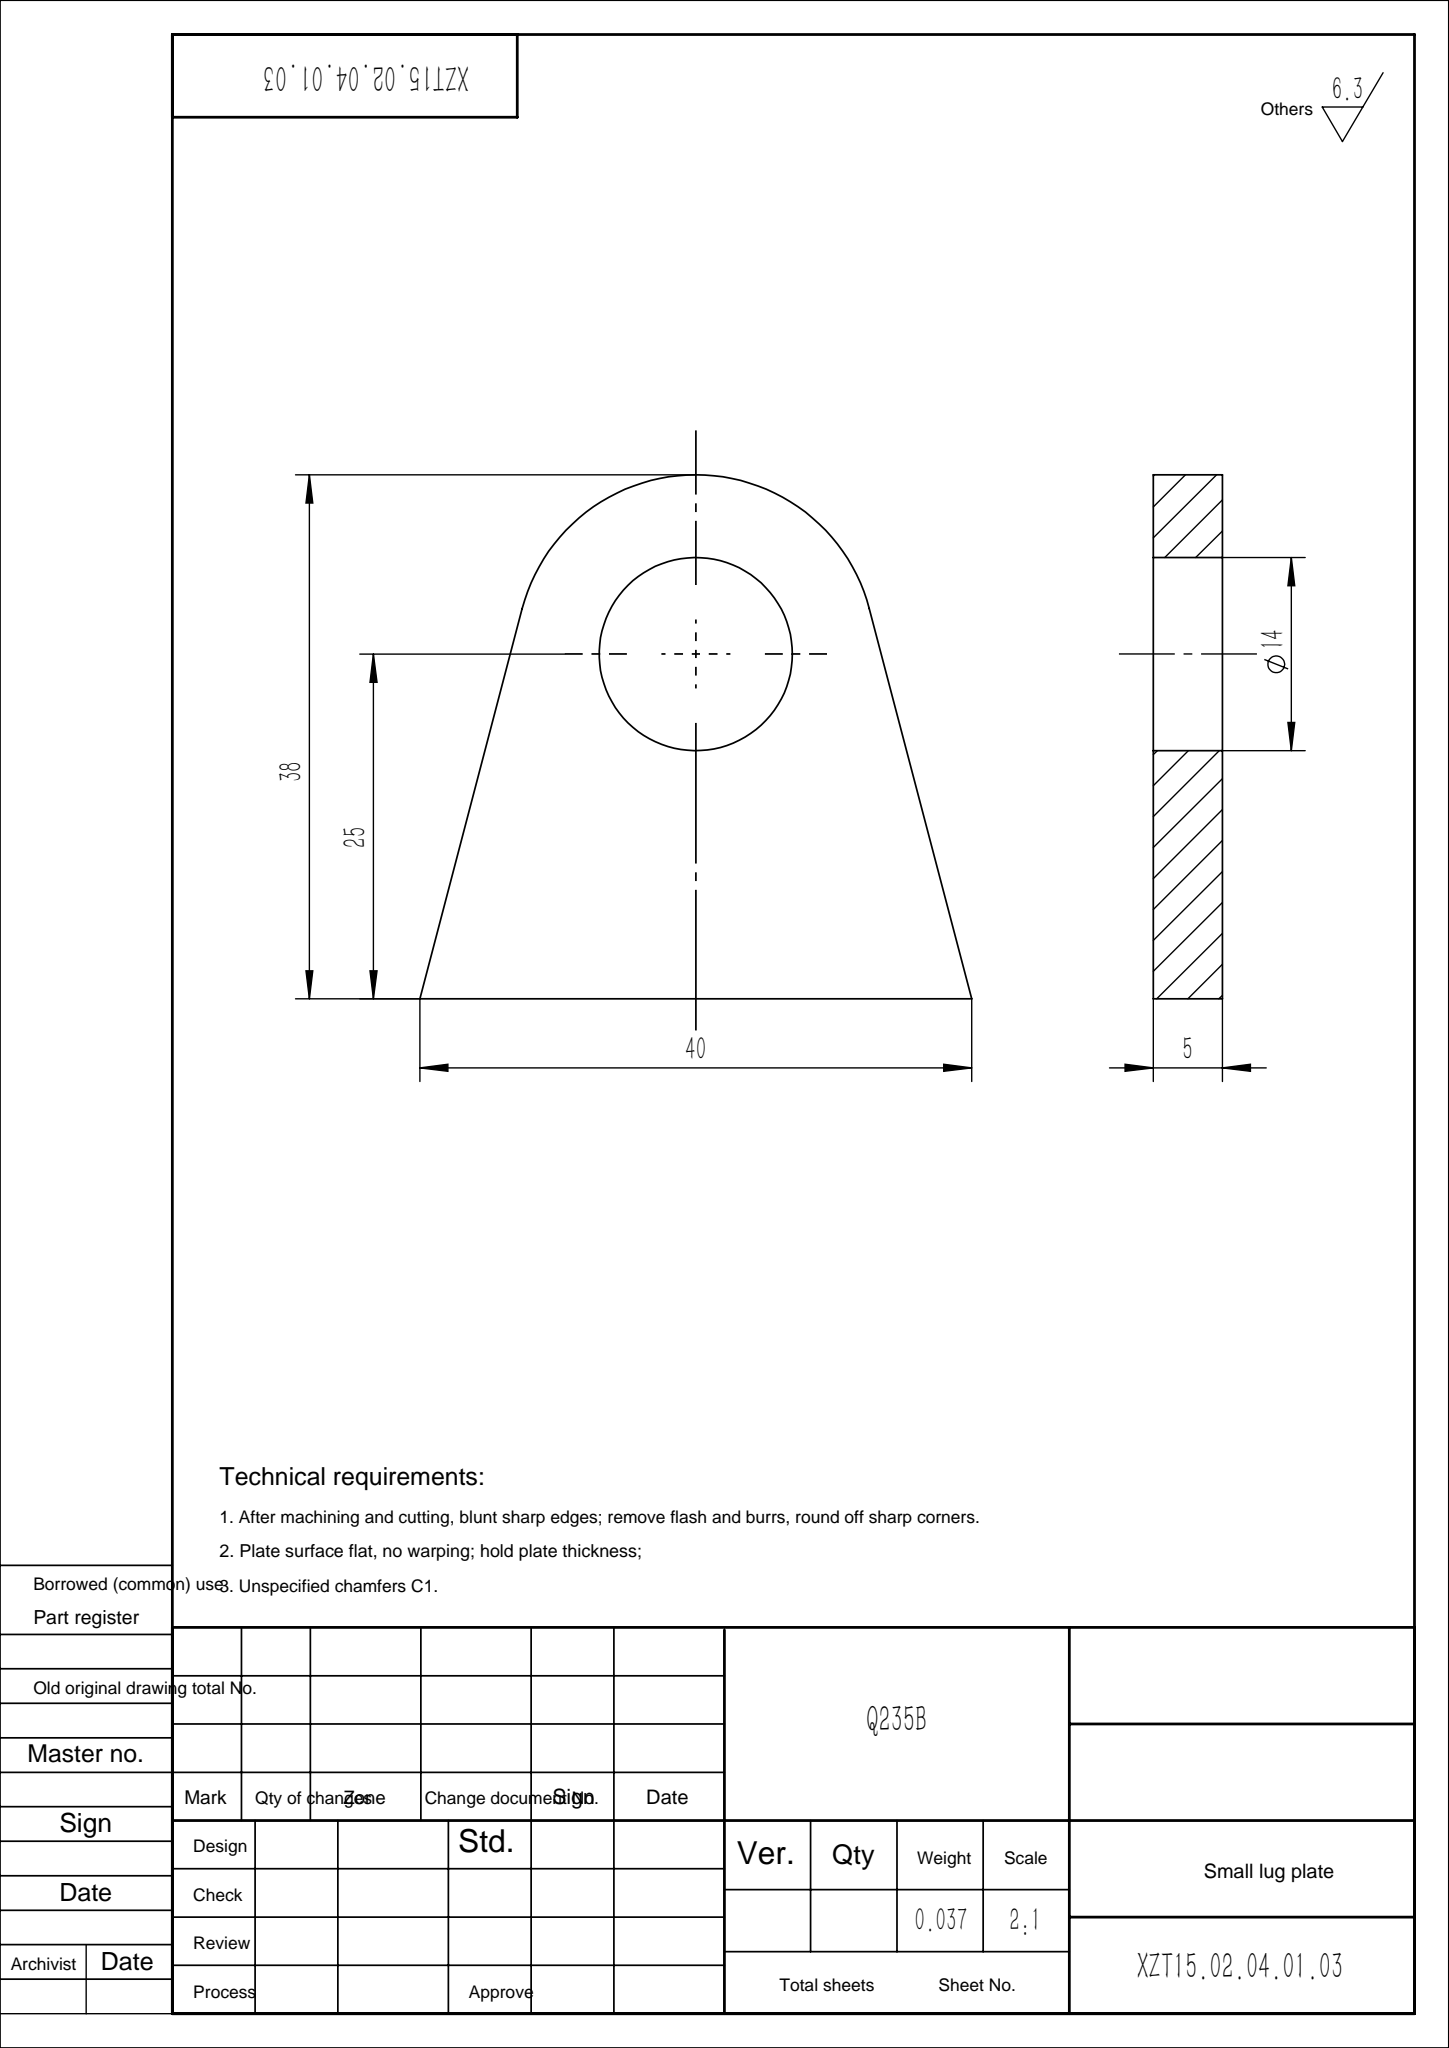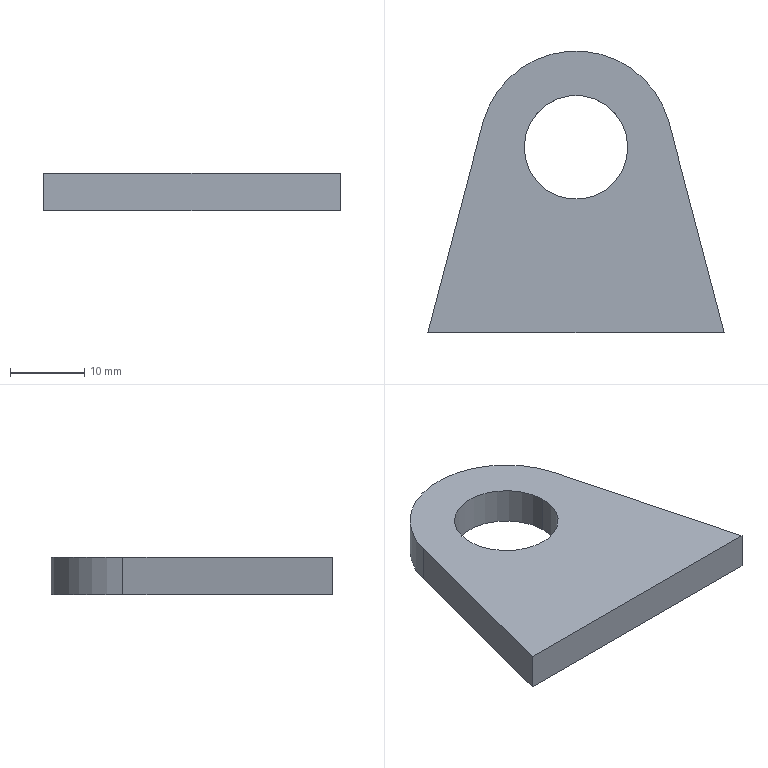Part | SolidWorks | features Extrusion 1 | 1 solid | 8 faces | box 40 x 38 x 5 mm | volume 4743 mm3 | plane 5 | cylinder 3 | commonest cylinder face diameters 14 x2 26 x1
STEP:
#1=CARTESIAN_POINT('',(-7.,25.,2.5));
#2=VERTEX_POINT('',#1);
#3=CARTESIAN_POINT('',(7.,25.,2.5));
#4=VERTEX_POINT('',#3);
#5=CARTESIAN_POINT('',(0.,25.,2.5));
#6=DIRECTION('',(0.,0.,1.));
#7=DIRECTION('',(1.,0.,0.));
#8=AXIS2_PLACEMENT_3D('',#5,#6,#7);
#9=CIRCLE('',#8,7.);
#10=EDGE_CURVE('',#2,#4,#9,.T.);
#11=ORIENTED_EDGE('',*,*,#10,.T.);
#12=CARTESIAN_POINT('',(7.,25.,-2.5));
#13=VERTEX_POINT('',#12);
#14=CARTESIAN_POINT('',(7.,25.,2.5));
#15=DIRECTION('',(0.,0.,-1.));
#16=VECTOR('',#15,1000.);
#17=LINE('',#14,#16);
#18=EDGE_CURVE('',#4,#13,#17,.T.);
#19=ORIENTED_EDGE('',*,*,#18,.T.);
#20=CARTESIAN_POINT('',(-7.,25.,-2.5));
#21=VERTEX_POINT('',#20);
#22=CARTESIAN_POINT('',(0.,25.,-2.5));
#23=DIRECTION('',(0.,0.,1.));
#24=DIRECTION('',(1.,0.,0.));
#25=AXIS2_PLACEMENT_3D('',#22,#23,#24);
#26=CIRCLE('',#25,7.);
#27=EDGE_CURVE('',#21,#13,#26,.T.);
#28=ORIENTED_EDGE('',*,*,#27,.F.);
#29=CARTESIAN_POINT('',(-7.,25.,2.5));
#30=DIRECTION('',(0.,0.,-1.));
#31=VECTOR('',#30,1000.);
#32=LINE('',#29,#31);
#33=EDGE_CURVE('',#2,#21,#32,.T.);
#34=ORIENTED_EDGE('',*,*,#33,.F.);
#35=EDGE_LOOP('',(#11,#19,#28,#34));
#36=FACE_OUTER_BOUND('',#35,.T.);
#37=CARTESIAN_POINT('',(0.,25.,2.5));
#38=DIRECTION('',(0.,0.,-1.));
#39=DIRECTION('',(-1.,0.,0.));
#40=AXIS2_PLACEMENT_3D('',#37,#38,#39);
#41=CYLINDRICAL_SURFACE('',#40,7.);
#42=ADVANCED_FACE('',(#36),#41,.F.);
#43=CARTESIAN_POINT('',(-12.574,28.299,2.5));
#44=VERTEX_POINT('',#43);
#45=CARTESIAN_POINT('',(-20.,0.,2.5));
#46=VERTEX_POINT('',#45);
#47=CARTESIAN_POINT('',(-20.,0.,2.5));
#48=DIRECTION('',(-0.2538,-0.9673,0.));
#49=VECTOR('',#48,1000.);
#50=LINE('',#47,#49);
#51=EDGE_CURVE('',#44,#46,#50,.T.);
#52=ORIENTED_EDGE('',*,*,#51,.T.);
#53=CARTESIAN_POINT('',(20.,0.,2.5));
#54=VERTEX_POINT('',#53);
#55=CARTESIAN_POINT('',(20.,0.,2.5));
#56=DIRECTION('',(1.,0.,0.));
#57=VECTOR('',#56,1000.);
#58=LINE('',#55,#57);
#59=EDGE_CURVE('',#46,#54,#58,.T.);
#60=ORIENTED_EDGE('',*,*,#59,.T.);
#61=CARTESIAN_POINT('',(12.574,28.299,2.5));
#62=VERTEX_POINT('',#61);
#63=CARTESIAN_POINT('',(20.,0.,2.5));
#64=DIRECTION('',(-0.2538,0.9673,0.));
#65=VECTOR('',#64,1000.);
#66=LINE('',#63,#65);
#67=EDGE_CURVE('',#54,#62,#66,.T.);
#68=ORIENTED_EDGE('',*,*,#67,.T.);
#69=CARTESIAN_POINT('',(0.,25.,2.5));
#70=DIRECTION('',(0.,0.,1.));
#71=DIRECTION('',(-1.,0.,0.));
#72=AXIS2_PLACEMENT_3D('',#69,#70,#71);
#73=CIRCLE('',#72,13.);
#74=EDGE_CURVE('',#62,#44,#73,.T.);
#75=ORIENTED_EDGE('',*,*,#74,.T.);
#76=EDGE_LOOP('',(#52,#60,#68,#75));
#77=FACE_OUTER_BOUND('',#76,.T.);
#78=ORIENTED_EDGE('',*,*,#10,.F.);
#79=CARTESIAN_POINT('',(0.,25.,2.5));
#80=DIRECTION('',(0.,0.,1.));
#81=DIRECTION('',(1.,0.,0.));
#82=AXIS2_PLACEMENT_3D('',#79,#80,#81);
#83=CIRCLE('',#82,7.);
#84=EDGE_CURVE('',#4,#2,#83,.T.);
#85=ORIENTED_EDGE('',*,*,#84,.F.);
#86=EDGE_LOOP('',(#78,#85));
#87=FACE_BOUND('',#86,.T.);
#88=CARTESIAN_POINT('',(0.,25.,2.5));
#89=DIRECTION('',(0.,0.,-1.));
#90=DIRECTION('',(-1.,0.,0.));
#91=AXIS2_PLACEMENT_3D('',#88,#89,#90);
#92=PLANE('',#91);
#93=ADVANCED_FACE('',(#77,#87),#92,.F.);
#94=CARTESIAN_POINT('',(-12.574,28.299,-2.5));
#95=VERTEX_POINT('',#94);
#96=CARTESIAN_POINT('',(-20.,0.,-2.5));
#97=VERTEX_POINT('',#96);
#98=CARTESIAN_POINT('',(-20.,0.,-2.5));
#99=DIRECTION('',(-0.2538,-0.9673,0.));
#100=VECTOR('',#99,1000.);
#101=LINE('',#98,#100);
#102=EDGE_CURVE('',#95,#97,#101,.T.);
#103=ORIENTED_EDGE('',*,*,#102,.F.);
#104=CARTESIAN_POINT('',(12.574,28.299,-2.5));
#105=VERTEX_POINT('',#104);
#106=CARTESIAN_POINT('',(0.,25.,-2.5));
#107=DIRECTION('',(0.,0.,1.));
#108=DIRECTION('',(-1.,0.,0.));
#109=AXIS2_PLACEMENT_3D('',#106,#107,#108);
#110=CIRCLE('',#109,13.);
#111=EDGE_CURVE('',#105,#95,#110,.T.);
#112=ORIENTED_EDGE('',*,*,#111,.F.);
#113=CARTESIAN_POINT('',(20.,0.,-2.5));
#114=VERTEX_POINT('',#113);
#115=CARTESIAN_POINT('',(20.,0.,-2.5));
#116=DIRECTION('',(-0.2538,0.9673,0.));
#117=VECTOR('',#116,1000.);
#118=LINE('',#115,#117);
#119=EDGE_CURVE('',#114,#105,#118,.T.);
#120=ORIENTED_EDGE('',*,*,#119,.F.);
#121=CARTESIAN_POINT('',(20.,0.,-2.5));
#122=DIRECTION('',(1.,0.,0.));
#123=VECTOR('',#122,1000.);
#124=LINE('',#121,#123);
#125=EDGE_CURVE('',#97,#114,#124,.T.);
#126=ORIENTED_EDGE('',*,*,#125,.F.);
#127=EDGE_LOOP('',(#103,#112,#120,#126));
#128=FACE_OUTER_BOUND('',#127,.T.);
#129=ORIENTED_EDGE('',*,*,#27,.T.);
#130=CARTESIAN_POINT('',(0.,25.,-2.5));
#131=DIRECTION('',(0.,0.,1.));
#132=DIRECTION('',(1.,0.,0.));
#133=AXIS2_PLACEMENT_3D('',#130,#131,#132);
#134=CIRCLE('',#133,7.);
#135=EDGE_CURVE('',#13,#21,#134,.T.);
#136=ORIENTED_EDGE('',*,*,#135,.T.);
#137=EDGE_LOOP('',(#129,#136));
#138=FACE_BOUND('',#137,.T.);
#139=CARTESIAN_POINT('',(0.,25.,-2.5));
#140=DIRECTION('',(0.,0.,-1.));
#141=DIRECTION('',(-1.,0.,0.));
#142=AXIS2_PLACEMENT_3D('',#139,#140,#141);
#143=PLANE('',#142);
#144=ADVANCED_FACE('',(#128,#138),#143,.T.);
#145=ORIENTED_EDGE('',*,*,#102,.T.);
#146=CARTESIAN_POINT('',(-20.,0.,2.5));
#147=DIRECTION('',(0.,0.,-1.));
#148=VECTOR('',#147,1000.);
#149=LINE('',#146,#148);
#150=EDGE_CURVE('',#46,#97,#149,.T.);
#151=ORIENTED_EDGE('',*,*,#150,.F.);
#152=ORIENTED_EDGE('',*,*,#51,.F.);
#153=CARTESIAN_POINT('',(-12.574,28.299,2.5));
#154=DIRECTION('',(0.,0.,-1.));
#155=VECTOR('',#154,1000.);
#156=LINE('',#153,#155);
#157=EDGE_CURVE('',#44,#95,#156,.T.);
#158=ORIENTED_EDGE('',*,*,#157,.T.);
#159=EDGE_LOOP('',(#145,#151,#152,#158));
#160=FACE_OUTER_BOUND('',#159,.T.);
#161=CARTESIAN_POINT('',(-20.,0.,2.5));
#162=DIRECTION('',(0.9673,-0.2538,0.));
#163=DIRECTION('',(0.2538,0.9673,0.));
#164=AXIS2_PLACEMENT_3D('',#161,#162,#163);
#165=PLANE('',#164);
#166=ADVANCED_FACE('',(#160),#165,.F.);
#167=ORIENTED_EDGE('',*,*,#125,.T.);
#168=CARTESIAN_POINT('',(20.,0.,2.5));
#169=DIRECTION('',(0.,0.,-1.));
#170=VECTOR('',#169,1000.);
#171=LINE('',#168,#170);
#172=EDGE_CURVE('',#54,#114,#171,.T.);
#173=ORIENTED_EDGE('',*,*,#172,.F.);
#174=ORIENTED_EDGE('',*,*,#59,.F.);
#175=ORIENTED_EDGE('',*,*,#150,.T.);
#176=EDGE_LOOP('',(#167,#173,#174,#175));
#177=FACE_OUTER_BOUND('',#176,.T.);
#178=CARTESIAN_POINT('',(20.,0.,2.5));
#179=DIRECTION('',(0.,1.,0.));
#180=DIRECTION('',(0.,0.,1.));
#181=AXIS2_PLACEMENT_3D('',#178,#179,#180);
#182=PLANE('',#181);
#183=ADVANCED_FACE('',(#177),#182,.F.);
#184=ORIENTED_EDGE('',*,*,#119,.T.);
#185=CARTESIAN_POINT('',(12.574,28.299,2.5));
#186=DIRECTION('',(0.,0.,-1.));
#187=VECTOR('',#186,1000.);
#188=LINE('',#185,#187);
#189=EDGE_CURVE('',#62,#105,#188,.T.);
#190=ORIENTED_EDGE('',*,*,#189,.F.);
#191=ORIENTED_EDGE('',*,*,#67,.F.);
#192=ORIENTED_EDGE('',*,*,#172,.T.);
#193=EDGE_LOOP('',(#184,#190,#191,#192));
#194=FACE_OUTER_BOUND('',#193,.T.);
#195=CARTESIAN_POINT('',(20.,0.,2.5));
#196=DIRECTION('',(-0.9673,-0.2538,0.));
#197=DIRECTION('',(0.2538,-0.9673,0.));
#198=AXIS2_PLACEMENT_3D('',#195,#196,#197);
#199=PLANE('',#198);
#200=ADVANCED_FACE('',(#194),#199,.F.);
#201=ORIENTED_EDGE('',*,*,#111,.T.);
#202=ORIENTED_EDGE('',*,*,#157,.F.);
#203=ORIENTED_EDGE('',*,*,#74,.F.);
#204=ORIENTED_EDGE('',*,*,#189,.T.);
#205=EDGE_LOOP('',(#201,#202,#203,#204));
#206=FACE_OUTER_BOUND('',#205,.T.);
#207=CARTESIAN_POINT('',(0.,25.,2.5));
#208=DIRECTION('',(0.,0.,-1.));
#209=DIRECTION('',(-1.,0.,0.));
#210=AXIS2_PLACEMENT_3D('',#207,#208,#209);
#211=CYLINDRICAL_SURFACE('',#210,13.);
#212=ADVANCED_FACE('',(#206),#211,.T.);
#213=ORIENTED_EDGE('',*,*,#18,.F.);
#214=ORIENTED_EDGE('',*,*,#84,.T.);
#215=ORIENTED_EDGE('',*,*,#33,.T.);
#216=ORIENTED_EDGE('',*,*,#135,.F.);
#217=EDGE_LOOP('',(#213,#214,#215,#216));
#218=FACE_OUTER_BOUND('',#217,.T.);
#219=CARTESIAN_POINT('',(0.,25.,2.5));
#220=DIRECTION('',(0.,0.,-1.));
#221=DIRECTION('',(-1.,0.,0.));
#222=AXIS2_PLACEMENT_3D('',#219,#220,#221);
#223=CYLINDRICAL_SURFACE('',#222,7.);
#224=ADVANCED_FACE('',(#218),#223,.F.);
#225=CLOSED_SHELL('',(#42,#93,#144,#166,#183,#200,#212,#224));
#226=MANIFOLD_SOLID_BREP('',#225);
#227=CARTESIAN_POINT('',(0.,0.,0.));
#228=DIRECTION('',(0.,0.,1.));
#229=DIRECTION('',(1.,0.,0.));
#230=AXIS2_PLACEMENT_3D('',#227,#228,#229);
#231=(LENGTH_UNIT()NAMED_UNIT(*)SI_UNIT(.MILLI.,.METRE.));
#232=UNCERTAINTY_MEASURE_WITH_UNIT(LENGTH_MEASURE(0.00001),#231,'','');
#233=(NAMED_UNIT(*)PLANE_ANGLE_UNIT()SI_UNIT($,.RADIAN.));
#234=(NAMED_UNIT(*)SI_UNIT($,.STERADIAN.)SOLID_ANGLE_UNIT());
#235=(GEOMETRIC_REPRESENTATION_CONTEXT(3)GLOBAL_UNCERTAINTY_ASSIGNED_CONTEXT((#232))GLOBAL_UNIT_ASSIGNED_CONTEXT((#231,#233,#234))REPRESENTATION_CONTEXT('',''));
#236=ADVANCED_BREP_SHAPE_REPRESENTATION('',(#226,#230),#235);